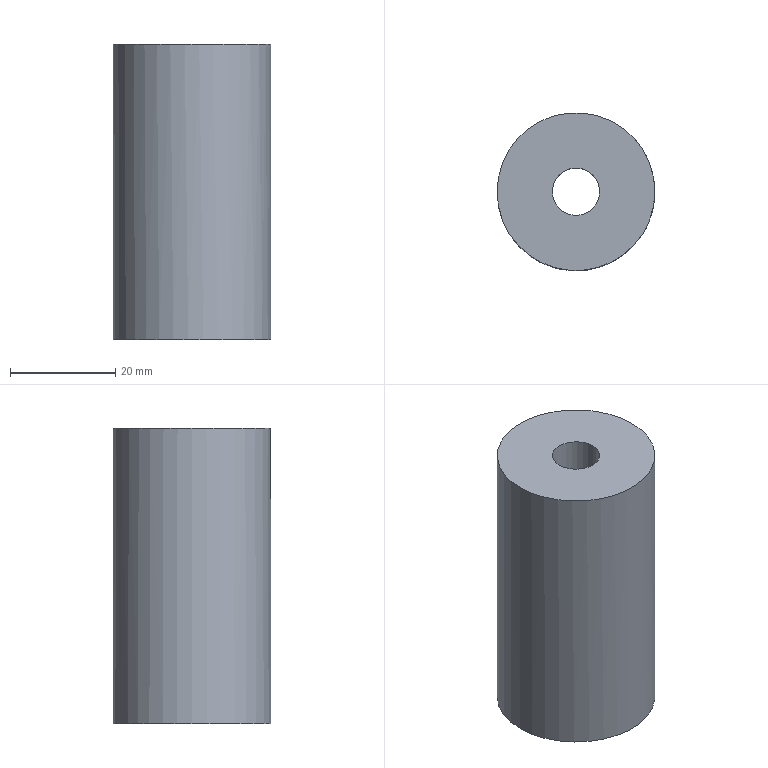Part | NX | features solid 2 | 1 solid | 6 faces | box 30 x 30 x 56.136 mm | volume 33218 mm3 | cylinder 3 | plane 3 | commonest cylinder face diameters 9 x1 14 x1 30 x1
STEP:
#1=CARTESIAN_POINT('',(-350.023,88.529,94.995));
#2=VERTEX_POINT('',#1);
#3=CARTESIAN_POINT('',(-335.023,88.529,94.995));
#4=DIRECTION('',(0.,0.,-1.));
#5=DIRECTION('',(-1.,0.,0.));
#6=AXIS2_PLACEMENT_3D('',#3,#4,#5);
#7=CIRCLE('',#6,15.);
#8=EDGE_CURVE('',#2,#2,#7,.T.);
#9=ORIENTED_EDGE('',*,*,#8,.F.);
#10=EDGE_LOOP('',(#9));
#11=FACE_BOUND('',#10,.T.);
#12=CARTESIAN_POINT('',(-320.023,88.529,151.131));
#13=VERTEX_POINT('',#12);
#14=CARTESIAN_POINT('',(-335.023,88.529,151.131));
#15=DIRECTION('',(0.,0.,-1.));
#16=DIRECTION('',(1.,0.,0.));
#17=AXIS2_PLACEMENT_3D('',#14,#15,#16);
#18=CIRCLE('',#17,15.);
#19=EDGE_CURVE('',#13,#13,#18,.T.);
#20=ORIENTED_EDGE('',*,*,#19,.T.);
#21=EDGE_LOOP('',(#20));
#22=FACE_BOUND('',#21,.T.);
#23=CARTESIAN_POINT('',(-335.023,88.529,86.));
#24=DIRECTION('',(-0.000000053,0.000000517,-1.));
#25=DIRECTION('',(0.,-1.,-0.000000517));
#26=AXIS2_PLACEMENT_3D('',#23,#24,#25);
#27=CYLINDRICAL_SURFACE('',#26,15.);
#28=ADVANCED_FACE('',(#11,#22),#27,.T.);
#29=CARTESIAN_POINT('',(-330.523,88.529,151.131));
#30=VERTEX_POINT('',#29);
#31=CARTESIAN_POINT('',(-335.023,88.529,151.131));
#32=DIRECTION('',(0.,0.,-1.));
#33=DIRECTION('',(1.,0.,0.));
#34=AXIS2_PLACEMENT_3D('',#31,#32,#33);
#35=CIRCLE('',#34,4.5);
#36=EDGE_CURVE('',#30,#30,#35,.F.);
#37=ORIENTED_EDGE('',*,*,#36,.T.);
#38=EDGE_LOOP('',(#37));
#39=FACE_BOUND('',#38,.T.);
#40=CARTESIAN_POINT('',(-339.523,88.529,126.998));
#41=VERTEX_POINT('',#40);
#42=CARTESIAN_POINT('',(-335.023,88.529,126.998));
#43=DIRECTION('',(0.000000053,-0.000000517,1.));
#44=DIRECTION('',(-1.,0.,0.000000053));
#45=AXIS2_PLACEMENT_3D('',#42,#43,#44);
#46=CIRCLE('',#45,4.5);
#47=EDGE_CURVE('',#41,#41,#46,.T.);
#48=ORIENTED_EDGE('',*,*,#47,.F.);
#49=EDGE_LOOP('',(#48));
#50=FACE_BOUND('',#49,.T.);
#51=CARTESIAN_POINT('',(-335.023,88.529,46.));
#52=DIRECTION('',(0.000000053,-0.000000517,1.));
#53=DIRECTION('',(0.,-1.,-0.000000517));
#54=AXIS2_PLACEMENT_3D('',#51,#52,#53);
#55=CYLINDRICAL_SURFACE('',#54,4.5);
#56=ADVANCED_FACE('',(#39,#50),#55,.F.);
#57=ORIENTED_EDGE('',*,*,#47,.T.);
#58=EDGE_LOOP('',(#57));
#59=FACE_BOUND('',#58,.T.);
#60=CARTESIAN_POINT('',(-342.023,88.529,126.998));
#61=VERTEX_POINT('',#60);
#62=CARTESIAN_POINT('',(-335.023,88.529,126.998));
#63=DIRECTION('',(0.000000053,-0.000000517,1.));
#64=DIRECTION('',(-1.,0.,0.000000053));
#65=AXIS2_PLACEMENT_3D('',#62,#63,#64);
#66=CIRCLE('',#65,7.);
#67=EDGE_CURVE('',#61,#61,#66,.T.);
#68=ORIENTED_EDGE('',*,*,#67,.F.);
#69=EDGE_LOOP('',(#68));
#70=FACE_BOUND('',#69,.T.);
#71=CARTESIAN_POINT('',(-457.523,261.529,126.998));
#72=DIRECTION('',(-0.000000053,0.000000517,-1.));
#73=DIRECTION('',(1.,0.,-0.000000053));
#74=AXIS2_PLACEMENT_3D('',#71,#72,#73);
#75=PLANE('',#74);
#76=ADVANCED_FACE('',(#59,#70),#75,.T.);
#77=CARTESIAN_POINT('',(-342.023,88.529,94.995));
#78=VERTEX_POINT('',#77);
#79=CARTESIAN_POINT('',(-335.023,88.529,94.995));
#80=DIRECTION('',(0.,0.,-1.));
#81=DIRECTION('',(-1.,0.,0.));
#82=AXIS2_PLACEMENT_3D('',#79,#80,#81);
#83=CIRCLE('',#82,7.);
#84=EDGE_CURVE('',#78,#78,#83,.F.);
#85=ORIENTED_EDGE('',*,*,#84,.F.);
#86=EDGE_LOOP('',(#85));
#87=FACE_BOUND('',#86,.T.);
#88=ORIENTED_EDGE('',*,*,#67,.T.);
#89=EDGE_LOOP('',(#88));
#90=FACE_BOUND('',#89,.T.);
#91=CARTESIAN_POINT('',(-335.023,88.529,88.));
#92=DIRECTION('',(0.000000053,-0.000000517,1.));
#93=DIRECTION('',(0.,-1.,-0.000000517));
#94=AXIS2_PLACEMENT_3D('',#91,#92,#93);
#95=CYLINDRICAL_SURFACE('',#94,7.);
#96=ADVANCED_FACE('',(#87,#90),#95,.F.);
#97=ORIENTED_EDGE('',*,*,#19,.F.);
#98=EDGE_LOOP('',(#97));
#99=FACE_BOUND('',#98,.T.);
#100=ORIENTED_EDGE('',*,*,#36,.F.);
#101=EDGE_LOOP('',(#100));
#102=FACE_BOUND('',#101,.T.);
#103=CARTESIAN_POINT('',(1449.977,94.59,151.131));
#104=DIRECTION('',(0.,0.,-1.));
#105=DIRECTION('',(0.,-1.,0.));
#106=AXIS2_PLACEMENT_3D('',#103,#104,#105);
#107=PLANE('',#106);
#108=ADVANCED_FACE('',(#99,#102),#107,.F.);
#109=ORIENTED_EDGE('',*,*,#8,.T.);
#110=EDGE_LOOP('',(#109));
#111=FACE_BOUND('',#110,.T.);
#112=ORIENTED_EDGE('',*,*,#84,.T.);
#113=EDGE_LOOP('',(#112));
#114=FACE_BOUND('',#113,.T.);
#115=CARTESIAN_POINT('',(-150.023,-16.972,94.995));
#116=DIRECTION('',(0.,0.,-1.));
#117=DIRECTION('',(-1.,0.,0.));
#118=AXIS2_PLACEMENT_3D('',#115,#116,#117);
#119=PLANE('',#118);
#120=ADVANCED_FACE('',(#111,#114),#119,.T.);
#121=CLOSED_SHELL('',(#28,#56,#76,#96,#108,#120));
#122=MANIFOLD_SOLID_BREP('',#121);
#123=(LENGTH_UNIT()NAMED_UNIT(*)SI_UNIT(.MILLI.,.METRE.));
#124=UNCERTAINTY_MEASURE_WITH_UNIT(LENGTH_MEASURE(0.00001),#123,'','');
#125=(NAMED_UNIT(*)PLANE_ANGLE_UNIT()SI_UNIT($,.RADIAN.));
#126=(NAMED_UNIT(*)SI_UNIT($,.STERADIAN.)SOLID_ANGLE_UNIT());
#127=(GEOMETRIC_REPRESENTATION_CONTEXT(3)GLOBAL_UNCERTAINTY_ASSIGNED_CONTEXT((#124))GLOBAL_UNIT_ASSIGNED_CONTEXT((#123,#125,#126))REPRESENTATION_CONTEXT('',''));
#128=ADVANCED_BREP_SHAPE_REPRESENTATION('',(#122),#127);